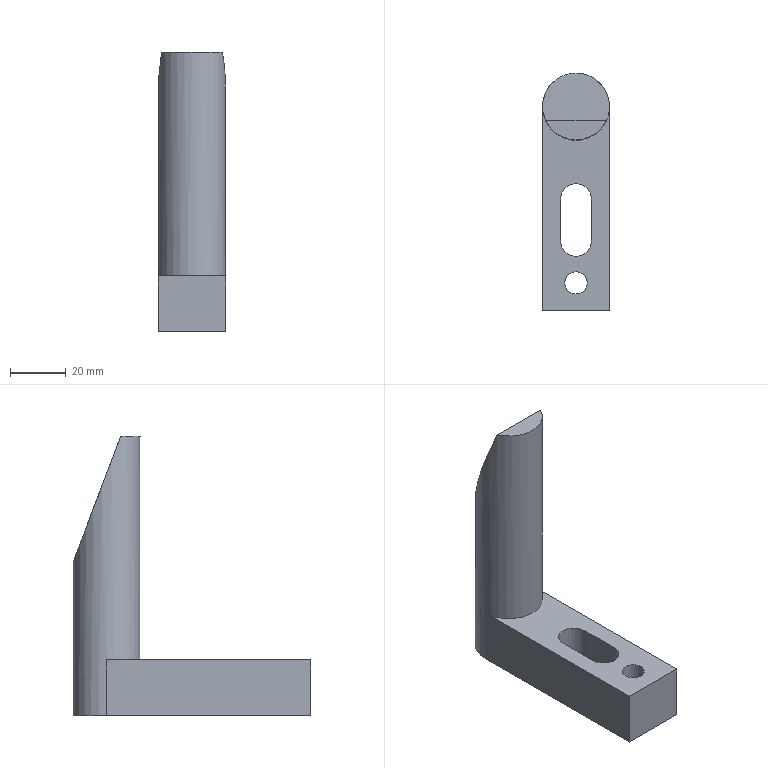Part | NX | features MAIN_BODY 2 | 1 solid | 13 faces | box 24 x 85 x 100 mm | volume 62724 mm3 | plane 9 | cylinder 4 | commonest cylinder face diameters 11 x2 8 x1 24 x1
STEP:
#1=CARTESIAN_POINT('',(728.,-535.,-95.));
#2=VERTEX_POINT('',#1);
#3=CARTESIAN_POINT('',(752.,-535.,-95.));
#4=VERTEX_POINT('',#3);
#5=CARTESIAN_POINT('',(740.,-535.,-95.));
#6=DIRECTION('',(0.,0.,-1.));
#7=DIRECTION('',(-1.,0.,0.));
#8=AXIS2_PLACEMENT_3D('',#5,#6,#7);
#9=CIRCLE('',#8,12.);
#10=EDGE_CURVE('',#2,#4,#9,.T.);
#11=ORIENTED_EDGE('',*,*,#10,.F.);
#12=CARTESIAN_POINT('',(728.,-535.,-75.));
#13=VERTEX_POINT('',#12);
#14=CARTESIAN_POINT('',(728.,-535.,-75.));
#15=DIRECTION('',(0.,0.,-1.));
#16=VECTOR('',#15,1000.);
#17=LINE('',#14,#16);
#18=EDGE_CURVE('',#13,#2,#17,.T.);
#19=ORIENTED_EDGE('',*,*,#18,.F.);
#20=CARTESIAN_POINT('',(752.,-535.,-75.));
#21=VERTEX_POINT('',#20);
#22=CARTESIAN_POINT('',(740.,-535.,-75.));
#23=DIRECTION('',(0.,0.,-1.));
#24=DIRECTION('',(-1.,0.,0.));
#25=AXIS2_PLACEMENT_3D('',#22,#23,#24);
#26=CIRCLE('',#25,12.);
#27=EDGE_CURVE('',#13,#21,#26,.F.);
#28=ORIENTED_EDGE('',*,*,#27,.T.);
#29=CARTESIAN_POINT('',(752.,-535.,-75.));
#30=DIRECTION('',(0.,0.,-1.));
#31=VECTOR('',#30,1000.);
#32=LINE('',#29,#31);
#33=EDGE_CURVE('',#21,#4,#32,.T.);
#34=ORIENTED_EDGE('',*,*,#33,.T.);
#35=EDGE_LOOP('',(#11,#19,#28,#34));
#36=FACE_BOUND('',#35,.T.);
#37=CARTESIAN_POINT('',(729.091,-540.,5.));
#38=VERTEX_POINT('',#37);
#39=CARTESIAN_POINT('',(750.909,-540.,5.));
#40=VERTEX_POINT('',#39);
#41=CARTESIAN_POINT('',(740.,-535.,-8.235));
#42=DIRECTION('',(0.,-0.9355,-0.3534));
#43=DIRECTION('',(0.,0.3534,-0.9355));
#44=AXIS2_PLACEMENT_3D('',#41,#42,#43);
#45=ELLIPSE('',#44,33.956,12.);
#46=EDGE_CURVE('',#38,#40,#45,.T.);
#47=ORIENTED_EDGE('',*,*,#46,.T.);
#48=CARTESIAN_POINT('',(740.,-535.,5.));
#49=DIRECTION('',(0.,0.,-1.));
#50=DIRECTION('',(-1.,0.,0.));
#51=AXIS2_PLACEMENT_3D('',#48,#49,#50);
#52=CIRCLE('',#51,12.);
#53=EDGE_CURVE('',#40,#38,#52,.T.);
#54=ORIENTED_EDGE('',*,*,#53,.T.);
#55=EDGE_LOOP('',(#47,#54));
#56=FACE_BOUND('',#55,.T.);
#57=CARTESIAN_POINT('',(740.,-535.,5.));
#58=DIRECTION('',(0.,0.,-1.));
#59=DIRECTION('',(1.,0.,0.));
#60=AXIS2_PLACEMENT_3D('',#57,#58,#59);
#61=CYLINDRICAL_SURFACE('',#60,12.);
#62=ADVANCED_FACE('',(#36,#56),#61,.T.);
#63=ORIENTED_EDGE('',*,*,#53,.F.);
#64=CARTESIAN_POINT('',(740.,-540.,5.));
#65=DIRECTION('',(1.,0.,0.));
#66=VECTOR('',#65,1000.);
#67=LINE('',#64,#66);
#68=EDGE_CURVE('',#38,#40,#67,.T.);
#69=ORIENTED_EDGE('',*,*,#68,.F.);
#70=EDGE_LOOP('',(#63,#69));
#71=FACE_BOUND('',#70,.T.);
#72=CARTESIAN_POINT('',(740.,-535.,5.));
#73=DIRECTION('',(0.,0.,1.));
#74=DIRECTION('',(-1.,0.,0.));
#75=AXIS2_PLACEMENT_3D('',#72,#73,#74);
#76=PLANE('',#75);
#77=ADVANCED_FACE('',(#71),#76,.T.);
#78=CARTESIAN_POINT('',(744.,-598.,-75.));
#79=VERTEX_POINT('',#78);
#80=CARTESIAN_POINT('',(740.,-598.,-75.));
#81=DIRECTION('',(0.,0.,1.));
#82=DIRECTION('',(1.,0.,0.));
#83=AXIS2_PLACEMENT_3D('',#80,#81,#82);
#84=CIRCLE('',#83,4.);
#85=EDGE_CURVE('',#79,#79,#84,.T.);
#86=ORIENTED_EDGE('',*,*,#85,.F.);
#87=EDGE_LOOP('',(#86));
#88=FACE_BOUND('',#87,.T.);
#89=CARTESIAN_POINT('',(745.5,-583.,-75.));
#90=VERTEX_POINT('',#89);
#91=CARTESIAN_POINT('',(745.5,-568.,-75.));
#92=VERTEX_POINT('',#91);
#93=CARTESIAN_POINT('',(745.5,-583.,-75.));
#94=DIRECTION('',(0.,1.,0.));
#95=VECTOR('',#94,1000.);
#96=LINE('',#93,#95);
#97=EDGE_CURVE('',#90,#92,#96,.T.);
#98=ORIENTED_EDGE('',*,*,#97,.F.);
#99=CARTESIAN_POINT('',(734.5,-583.,-75.));
#100=VERTEX_POINT('',#99);
#101=CARTESIAN_POINT('',(740.,-583.,-75.));
#102=DIRECTION('',(0.,0.,-1.));
#103=DIRECTION('',(-1.,0.,0.));
#104=AXIS2_PLACEMENT_3D('',#101,#102,#103);
#105=CIRCLE('',#104,5.5);
#106=EDGE_CURVE('',#90,#100,#105,.T.);
#107=ORIENTED_EDGE('',*,*,#106,.T.);
#108=CARTESIAN_POINT('',(734.5,-568.,-75.));
#109=VERTEX_POINT('',#108);
#110=CARTESIAN_POINT('',(734.5,-583.,-75.));
#111=DIRECTION('',(0.,1.,0.));
#112=VECTOR('',#111,1000.);
#113=LINE('',#110,#112);
#114=EDGE_CURVE('',#100,#109,#113,.T.);
#115=ORIENTED_EDGE('',*,*,#114,.T.);
#116=CARTESIAN_POINT('',(740.,-568.,-75.));
#117=DIRECTION('',(0.,0.,-1.));
#118=DIRECTION('',(-1.,0.,0.));
#119=AXIS2_PLACEMENT_3D('',#116,#117,#118);
#120=CIRCLE('',#119,5.5);
#121=EDGE_CURVE('',#109,#92,#120,.T.);
#122=ORIENTED_EDGE('',*,*,#121,.T.);
#123=EDGE_LOOP('',(#98,#107,#115,#122));
#124=FACE_BOUND('',#123,.T.);
#125=CARTESIAN_POINT('',(728.,-608.,-75.));
#126=VERTEX_POINT('',#125);
#127=CARTESIAN_POINT('',(728.,-623.,-75.));
#128=DIRECTION('',(0.,1.,0.));
#129=VECTOR('',#128,1000.);
#130=LINE('',#127,#129);
#131=EDGE_CURVE('',#126,#13,#130,.T.);
#132=ORIENTED_EDGE('',*,*,#131,.F.);
#133=CARTESIAN_POINT('',(752.,-608.,-75.));
#134=VERTEX_POINT('',#133);
#135=CARTESIAN_POINT('',(752.,-608.,-75.));
#136=DIRECTION('',(-1.,0.,0.));
#137=VECTOR('',#136,1000.);
#138=LINE('',#135,#137);
#139=EDGE_CURVE('',#134,#126,#138,.T.);
#140=ORIENTED_EDGE('',*,*,#139,.F.);
#141=CARTESIAN_POINT('',(752.,-535.,-75.));
#142=DIRECTION('',(0.,-1.,0.));
#143=VECTOR('',#142,1000.);
#144=LINE('',#141,#143);
#145=EDGE_CURVE('',#21,#134,#144,.T.);
#146=ORIENTED_EDGE('',*,*,#145,.F.);
#147=ORIENTED_EDGE('',*,*,#27,.F.);
#148=EDGE_LOOP('',(#132,#140,#146,#147));
#149=FACE_BOUND('',#148,.T.);
#150=CARTESIAN_POINT('',(752.,-535.,-75.));
#151=DIRECTION('',(0.,0.,1.));
#152=DIRECTION('',(-1.,0.,0.));
#153=AXIS2_PLACEMENT_3D('',#150,#151,#152);
#154=PLANE('',#153);
#155=ADVANCED_FACE('',(#88,#124,#149),#154,.T.);
#156=CARTESIAN_POINT('',(752.,-608.,-95.));
#157=VERTEX_POINT('',#156);
#158=CARTESIAN_POINT('',(752.,-535.,-95.));
#159=DIRECTION('',(0.,-1.,0.));
#160=VECTOR('',#159,1000.);
#161=LINE('',#158,#160);
#162=EDGE_CURVE('',#4,#157,#161,.T.);
#163=ORIENTED_EDGE('',*,*,#162,.F.);
#164=ORIENTED_EDGE('',*,*,#33,.F.);
#165=ORIENTED_EDGE('',*,*,#145,.T.);
#166=CARTESIAN_POINT('',(752.,-608.,-75.));
#167=DIRECTION('',(0.,0.,-1.));
#168=VECTOR('',#167,1000.);
#169=LINE('',#166,#168);
#170=EDGE_CURVE('',#134,#157,#169,.T.);
#171=ORIENTED_EDGE('',*,*,#170,.T.);
#172=EDGE_LOOP('',(#163,#164,#165,#171));
#173=FACE_BOUND('',#172,.T.);
#174=CARTESIAN_POINT('',(752.,-535.,-75.));
#175=DIRECTION('',(-1.,0.,0.));
#176=DIRECTION('',(0.,1.,0.));
#177=AXIS2_PLACEMENT_3D('',#174,#175,#176);
#178=PLANE('',#177);
#179=ADVANCED_FACE('',(#173),#178,.F.);
#180=CARTESIAN_POINT('',(728.,-608.,-95.));
#181=VERTEX_POINT('',#180);
#182=CARTESIAN_POINT('',(752.,-608.,-95.));
#183=DIRECTION('',(-1.,0.,0.));
#184=VECTOR('',#183,1000.);
#185=LINE('',#182,#184);
#186=EDGE_CURVE('',#157,#181,#185,.T.);
#187=ORIENTED_EDGE('',*,*,#186,.F.);
#188=ORIENTED_EDGE('',*,*,#170,.F.);
#189=ORIENTED_EDGE('',*,*,#139,.T.);
#190=CARTESIAN_POINT('',(728.,-608.,-75.));
#191=DIRECTION('',(0.,0.,-1.));
#192=VECTOR('',#191,1000.);
#193=LINE('',#190,#192);
#194=EDGE_CURVE('',#126,#181,#193,.T.);
#195=ORIENTED_EDGE('',*,*,#194,.T.);
#196=EDGE_LOOP('',(#187,#188,#189,#195));
#197=FACE_BOUND('',#196,.T.);
#198=CARTESIAN_POINT('',(752.,-608.,-75.));
#199=DIRECTION('',(0.,1.,0.));
#200=DIRECTION('',(0.,0.,1.));
#201=AXIS2_PLACEMENT_3D('',#198,#199,#200);
#202=PLANE('',#201);
#203=ADVANCED_FACE('',(#197),#202,.F.);
#204=CARTESIAN_POINT('',(728.,-623.,-95.));
#205=DIRECTION('',(0.,1.,0.));
#206=VECTOR('',#205,1000.);
#207=LINE('',#204,#206);
#208=EDGE_CURVE('',#181,#2,#207,.T.);
#209=ORIENTED_EDGE('',*,*,#208,.F.);
#210=ORIENTED_EDGE('',*,*,#194,.F.);
#211=ORIENTED_EDGE('',*,*,#131,.T.);
#212=ORIENTED_EDGE('',*,*,#18,.T.);
#213=EDGE_LOOP('',(#209,#210,#211,#212));
#214=FACE_BOUND('',#213,.T.);
#215=CARTESIAN_POINT('',(728.,-623.,-75.));
#216=DIRECTION('',(1.,0.,0.));
#217=DIRECTION('',(0.,-1.,0.));
#218=AXIS2_PLACEMENT_3D('',#215,#216,#217);
#219=PLANE('',#218);
#220=ADVANCED_FACE('',(#214),#219,.F.);
#221=CARTESIAN_POINT('',(744.,-598.,-95.));
#222=VERTEX_POINT('',#221);
#223=CARTESIAN_POINT('',(740.,-598.,-95.));
#224=DIRECTION('',(0.,0.,1.));
#225=DIRECTION('',(1.,0.,0.));
#226=AXIS2_PLACEMENT_3D('',#223,#224,#225);
#227=CIRCLE('',#226,4.);
#228=EDGE_CURVE('',#222,#222,#227,.T.);
#229=ORIENTED_EDGE('',*,*,#228,.T.);
#230=EDGE_LOOP('',(#229));
#231=FACE_BOUND('',#230,.T.);
#232=CARTESIAN_POINT('',(734.5,-568.,-95.));
#233=VERTEX_POINT('',#232);
#234=CARTESIAN_POINT('',(745.5,-568.,-95.));
#235=VERTEX_POINT('',#234);
#236=CARTESIAN_POINT('',(740.,-568.,-95.));
#237=DIRECTION('',(0.,0.,-1.));
#238=DIRECTION('',(-1.,0.,0.));
#239=AXIS2_PLACEMENT_3D('',#236,#237,#238);
#240=CIRCLE('',#239,5.5);
#241=EDGE_CURVE('',#233,#235,#240,.T.);
#242=ORIENTED_EDGE('',*,*,#241,.F.);
#243=CARTESIAN_POINT('',(734.5,-583.,-95.));
#244=VERTEX_POINT('',#243);
#245=CARTESIAN_POINT('',(734.5,-598.,-95.));
#246=DIRECTION('',(0.,1.,0.));
#247=VECTOR('',#246,1000.);
#248=LINE('',#245,#247);
#249=EDGE_CURVE('',#244,#233,#248,.T.);
#250=ORIENTED_EDGE('',*,*,#249,.F.);
#251=CARTESIAN_POINT('',(745.5,-583.,-95.));
#252=VERTEX_POINT('',#251);
#253=CARTESIAN_POINT('',(740.,-583.,-95.));
#254=DIRECTION('',(0.,0.,-1.));
#255=DIRECTION('',(-1.,0.,0.));
#256=AXIS2_PLACEMENT_3D('',#253,#254,#255);
#257=CIRCLE('',#256,5.5);
#258=EDGE_CURVE('',#252,#244,#257,.T.);
#259=ORIENTED_EDGE('',*,*,#258,.F.);
#260=CARTESIAN_POINT('',(745.5,-598.,-95.));
#261=DIRECTION('',(0.,1.,0.));
#262=VECTOR('',#261,1000.);
#263=LINE('',#260,#262);
#264=EDGE_CURVE('',#252,#235,#263,.T.);
#265=ORIENTED_EDGE('',*,*,#264,.T.);
#266=EDGE_LOOP('',(#242,#250,#259,#265));
#267=FACE_BOUND('',#266,.T.);
#268=ORIENTED_EDGE('',*,*,#162,.T.);
#269=ORIENTED_EDGE('',*,*,#186,.T.);
#270=ORIENTED_EDGE('',*,*,#208,.T.);
#271=ORIENTED_EDGE('',*,*,#10,.T.);
#272=EDGE_LOOP('',(#268,#269,#270,#271));
#273=FACE_BOUND('',#272,.T.);
#274=CARTESIAN_POINT('',(752.,-535.,-95.));
#275=DIRECTION('',(0.,0.,1.));
#276=DIRECTION('',(-1.,0.,0.));
#277=AXIS2_PLACEMENT_3D('',#274,#275,#276);
#278=PLANE('',#277);
#279=ADVANCED_FACE('',(#231,#267,#273),#278,.F.);
#280=ORIENTED_EDGE('',*,*,#68,.T.);
#281=ORIENTED_EDGE('',*,*,#46,.F.);
#282=EDGE_LOOP('',(#280,#281));
#283=FACE_BOUND('',#282,.T.);
#284=CARTESIAN_POINT('',(811.5,-540.,5.));
#285=DIRECTION('',(0.,0.9355,0.3534));
#286=DIRECTION('',(0.,-0.3534,0.9355));
#287=AXIS2_PLACEMENT_3D('',#284,#285,#286);
#288=PLANE('',#287);
#289=ADVANCED_FACE('',(#283),#288,.T.);
#290=ORIENTED_EDGE('',*,*,#97,.T.);
#291=CARTESIAN_POINT('',(745.5,-568.,-75.));
#292=DIRECTION('',(0.,0.,1.));
#293=VECTOR('',#292,1000.);
#294=LINE('',#291,#293);
#295=EDGE_CURVE('',#235,#92,#294,.T.);
#296=ORIENTED_EDGE('',*,*,#295,.F.);
#297=ORIENTED_EDGE('',*,*,#264,.F.);
#298=CARTESIAN_POINT('',(745.5,-583.,-75.));
#299=DIRECTION('',(0.,0.,1.));
#300=VECTOR('',#299,1000.);
#301=LINE('',#298,#300);
#302=EDGE_CURVE('',#252,#90,#301,.T.);
#303=ORIENTED_EDGE('',*,*,#302,.T.);
#304=EDGE_LOOP('',(#290,#296,#297,#303));
#305=FACE_BOUND('',#304,.T.);
#306=CARTESIAN_POINT('',(745.5,-583.,-75.));
#307=DIRECTION('',(1.,0.,0.));
#308=DIRECTION('',(0.,0.,1.));
#309=AXIS2_PLACEMENT_3D('',#306,#307,#308);
#310=PLANE('',#309);
#311=ADVANCED_FACE('',(#305),#310,.F.);
#312=ORIENTED_EDGE('',*,*,#106,.F.);
#313=ORIENTED_EDGE('',*,*,#302,.F.);
#314=ORIENTED_EDGE('',*,*,#258,.T.);
#315=CARTESIAN_POINT('',(734.5,-583.,-75.));
#316=DIRECTION('',(0.,0.,1.));
#317=VECTOR('',#316,1000.);
#318=LINE('',#315,#317);
#319=EDGE_CURVE('',#244,#100,#318,.T.);
#320=ORIENTED_EDGE('',*,*,#319,.T.);
#321=EDGE_LOOP('',(#312,#313,#314,#320));
#322=FACE_BOUND('',#321,.T.);
#323=CARTESIAN_POINT('',(740.,-583.,-75.));
#324=DIRECTION('',(0.,0.,1.));
#325=DIRECTION('',(-1.,0.,0.));
#326=AXIS2_PLACEMENT_3D('',#323,#324,#325);
#327=CYLINDRICAL_SURFACE('',#326,5.5);
#328=ADVANCED_FACE('',(#322),#327,.F.);
#329=ORIENTED_EDGE('',*,*,#114,.F.);
#330=ORIENTED_EDGE('',*,*,#319,.F.);
#331=ORIENTED_EDGE('',*,*,#249,.T.);
#332=CARTESIAN_POINT('',(734.5,-568.,-75.));
#333=DIRECTION('',(0.,0.,1.));
#334=VECTOR('',#333,1000.);
#335=LINE('',#332,#334);
#336=EDGE_CURVE('',#233,#109,#335,.T.);
#337=ORIENTED_EDGE('',*,*,#336,.T.);
#338=EDGE_LOOP('',(#329,#330,#331,#337));
#339=FACE_BOUND('',#338,.T.);
#340=CARTESIAN_POINT('',(734.5,-583.,-75.));
#341=DIRECTION('',(-1.,0.,0.));
#342=DIRECTION('',(0.,0.,-1.));
#343=AXIS2_PLACEMENT_3D('',#340,#341,#342);
#344=PLANE('',#343);
#345=ADVANCED_FACE('',(#339),#344,.F.);
#346=ORIENTED_EDGE('',*,*,#121,.F.);
#347=ORIENTED_EDGE('',*,*,#336,.F.);
#348=ORIENTED_EDGE('',*,*,#241,.T.);
#349=ORIENTED_EDGE('',*,*,#295,.T.);
#350=EDGE_LOOP('',(#346,#347,#348,#349));
#351=FACE_BOUND('',#350,.T.);
#352=CARTESIAN_POINT('',(740.,-568.,-75.));
#353=DIRECTION('',(0.,0.,1.));
#354=DIRECTION('',(-1.,0.,0.));
#355=AXIS2_PLACEMENT_3D('',#352,#353,#354);
#356=CYLINDRICAL_SURFACE('',#355,5.5);
#357=ADVANCED_FACE('',(#351),#356,.F.);
#358=ORIENTED_EDGE('',*,*,#228,.F.);
#359=EDGE_LOOP('',(#358));
#360=FACE_BOUND('',#359,.T.);
#361=ORIENTED_EDGE('',*,*,#85,.T.);
#362=EDGE_LOOP('',(#361));
#363=FACE_BOUND('',#362,.T.);
#364=CARTESIAN_POINT('',(740.,-598.,-75.));
#365=DIRECTION('',(0.,0.,-1.));
#366=DIRECTION('',(1.,0.,0.));
#367=AXIS2_PLACEMENT_3D('',#364,#365,#366);
#368=CYLINDRICAL_SURFACE('',#367,4.);
#369=ADVANCED_FACE('',(#360,#363),#368,.F.);
#370=CLOSED_SHELL('',(#62,#77,#155,#179,#203,#220,#279,#289,#311,#328,#345,#357,#369));
#371=MANIFOLD_SOLID_BREP('',#370);
#372=(LENGTH_UNIT()NAMED_UNIT(*)SI_UNIT(.MILLI.,.METRE.));
#373=UNCERTAINTY_MEASURE_WITH_UNIT(LENGTH_MEASURE(0.00001),#372,'','');
#374=(NAMED_UNIT(*)PLANE_ANGLE_UNIT()SI_UNIT($,.RADIAN.));
#375=(NAMED_UNIT(*)SI_UNIT($,.STERADIAN.)SOLID_ANGLE_UNIT());
#376=(GEOMETRIC_REPRESENTATION_CONTEXT(3)GLOBAL_UNCERTAINTY_ASSIGNED_CONTEXT((#373))GLOBAL_UNIT_ASSIGNED_CONTEXT((#372,#374,#375))REPRESENTATION_CONTEXT('',''));
#377=ADVANCED_BREP_SHAPE_REPRESENTATION('',(#371),#376);